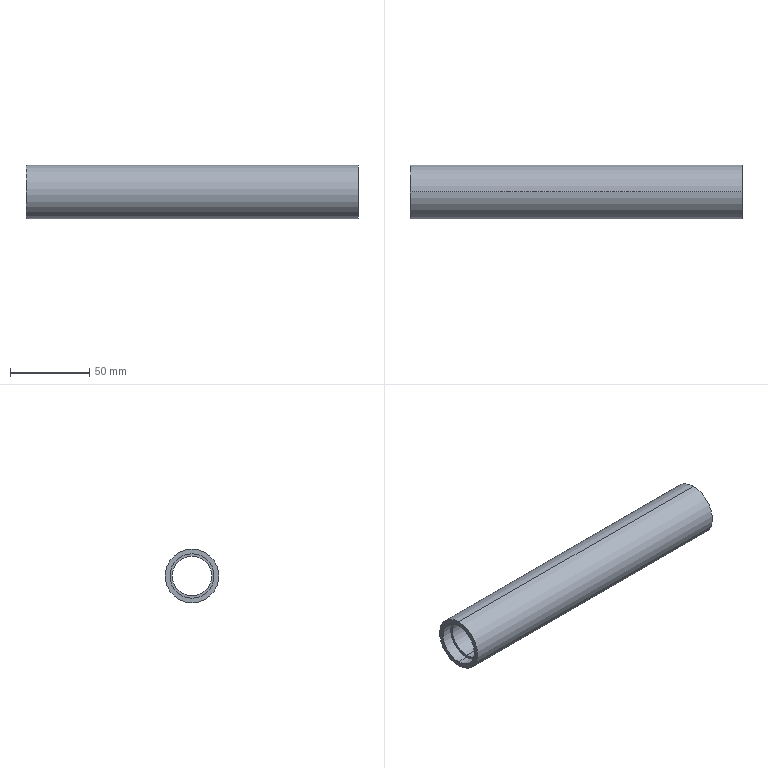Part | SolidWorks | features Revolution 1 | 1 solid | 12 faces | box 210 x 34 x 34 mm | volume 85831 mm3 | cylinder 8 | plane 4 | commonest cylinder face diameters 28 x4 25 x2 34 x2
STEP:
#1=CARTESIAN_POINT('',(98.,0.,-12.5));
#2=VERTEX_POINT('',#1);
#3=CARTESIAN_POINT('',(98.,0.,12.5));
#4=VERTEX_POINT('',#3);
#5=CARTESIAN_POINT('',(98.,0.,0.));
#6=DIRECTION('',(-1.,0.,0.));
#7=DIRECTION('',(0.,0.,1.));
#8=AXIS2_PLACEMENT_3D('',#5,#6,#7);
#9=CIRCLE('',#8,12.5);
#10=EDGE_CURVE('',#2,#4,#9,.T.);
#11=ORIENTED_EDGE('',*,*,#10,.F.);
#12=CARTESIAN_POINT('',(-98.,0.,-12.5));
#13=VERTEX_POINT('',#12);
#14=CARTESIAN_POINT('',(0.,0.,-12.5));
#15=DIRECTION('',(-1.,0.,0.));
#16=VECTOR('',#15,1000.);
#17=LINE('',#14,#16);
#18=EDGE_CURVE('',#2,#13,#17,.T.);
#19=ORIENTED_EDGE('',*,*,#18,.T.);
#20=CARTESIAN_POINT('',(-98.,0.,12.5));
#21=VERTEX_POINT('',#20);
#22=CARTESIAN_POINT('',(-98.,0.,0.));
#23=DIRECTION('',(-1.,0.,0.));
#24=DIRECTION('',(0.,0.,1.));
#25=AXIS2_PLACEMENT_3D('',#22,#23,#24);
#26=CIRCLE('',#25,12.5);
#27=EDGE_CURVE('',#13,#21,#26,.T.);
#28=ORIENTED_EDGE('',*,*,#27,.T.);
#29=CARTESIAN_POINT('',(0.,0.,12.5));
#30=DIRECTION('',(-1.,0.,0.));
#31=VECTOR('',#30,1000.);
#32=LINE('',#29,#31);
#33=EDGE_CURVE('',#4,#21,#32,.T.);
#34=ORIENTED_EDGE('',*,*,#33,.F.);
#35=EDGE_LOOP('',(#11,#19,#28,#34));
#36=FACE_OUTER_BOUND('',#35,.T.);
#37=CARTESIAN_POINT('',(0.,0.,0.));
#38=DIRECTION('',(-1.,0.,0.));
#39=DIRECTION('',(0.,0.,1.));
#40=AXIS2_PLACEMENT_3D('',#37,#38,#39);
#41=CYLINDRICAL_SURFACE('',#40,12.5);
#42=ADVANCED_FACE('',(#36),#41,.F.);
#43=CARTESIAN_POINT('',(105.,0.,-14.));
#44=VERTEX_POINT('',#43);
#45=CARTESIAN_POINT('',(105.,0.,14.));
#46=VERTEX_POINT('',#45);
#47=CARTESIAN_POINT('',(105.,0.,0.));
#48=DIRECTION('',(-1.,0.,0.));
#49=DIRECTION('',(0.,0.,1.));
#50=AXIS2_PLACEMENT_3D('',#47,#48,#49);
#51=CIRCLE('',#50,14.);
#52=EDGE_CURVE('',#44,#46,#51,.T.);
#53=ORIENTED_EDGE('',*,*,#52,.F.);
#54=CARTESIAN_POINT('',(98.,0.,-14.));
#55=VERTEX_POINT('',#54);
#56=CARTESIAN_POINT('',(0.,0.,-14.));
#57=DIRECTION('',(-1.,0.,0.));
#58=VECTOR('',#57,1000.);
#59=LINE('',#56,#58);
#60=EDGE_CURVE('',#44,#55,#59,.T.);
#61=ORIENTED_EDGE('',*,*,#60,.T.);
#62=CARTESIAN_POINT('',(98.,0.,14.));
#63=VERTEX_POINT('',#62);
#64=CARTESIAN_POINT('',(98.,0.,0.));
#65=DIRECTION('',(-1.,0.,0.));
#66=DIRECTION('',(0.,0.,1.));
#67=AXIS2_PLACEMENT_3D('',#64,#65,#66);
#68=CIRCLE('',#67,14.);
#69=EDGE_CURVE('',#55,#63,#68,.T.);
#70=ORIENTED_EDGE('',*,*,#69,.T.);
#71=CARTESIAN_POINT('',(0.,0.,14.));
#72=DIRECTION('',(-1.,0.,0.));
#73=VECTOR('',#72,1000.);
#74=LINE('',#71,#73);
#75=EDGE_CURVE('',#46,#63,#74,.T.);
#76=ORIENTED_EDGE('',*,*,#75,.F.);
#77=EDGE_LOOP('',(#53,#61,#70,#76));
#78=FACE_OUTER_BOUND('',#77,.T.);
#79=CARTESIAN_POINT('',(0.,0.,0.));
#80=DIRECTION('',(-1.,0.,0.));
#81=DIRECTION('',(0.,0.,1.));
#82=AXIS2_PLACEMENT_3D('',#79,#80,#81);
#83=CYLINDRICAL_SURFACE('',#82,14.);
#84=ADVANCED_FACE('',(#78),#83,.F.);
#85=CARTESIAN_POINT('',(105.,0.,17.));
#86=VERTEX_POINT('',#85);
#87=CARTESIAN_POINT('',(105.,0.,-17.));
#88=VERTEX_POINT('',#87);
#89=CARTESIAN_POINT('',(105.,0.,0.));
#90=DIRECTION('',(-1.,0.,0.));
#91=DIRECTION('',(0.,0.,1.));
#92=AXIS2_PLACEMENT_3D('',#89,#90,#91);
#93=CIRCLE('',#92,17.);
#94=EDGE_CURVE('',#86,#88,#93,.T.);
#95=ORIENTED_EDGE('',*,*,#94,.T.);
#96=CARTESIAN_POINT('',(-105.,0.,-17.));
#97=VERTEX_POINT('',#96);
#98=CARTESIAN_POINT('',(0.,0.,-17.));
#99=DIRECTION('',(-1.,0.,0.));
#100=VECTOR('',#99,1000.);
#101=LINE('',#98,#100);
#102=EDGE_CURVE('',#88,#97,#101,.T.);
#103=ORIENTED_EDGE('',*,*,#102,.T.);
#104=CARTESIAN_POINT('',(-105.,0.,17.));
#105=VERTEX_POINT('',#104);
#106=CARTESIAN_POINT('',(-105.,0.,0.));
#107=DIRECTION('',(-1.,0.,0.));
#108=DIRECTION('',(0.,0.,1.));
#109=AXIS2_PLACEMENT_3D('',#106,#107,#108);
#110=CIRCLE('',#109,17.);
#111=EDGE_CURVE('',#105,#97,#110,.T.);
#112=ORIENTED_EDGE('',*,*,#111,.F.);
#113=CARTESIAN_POINT('',(0.,0.,17.));
#114=DIRECTION('',(-1.,0.,0.));
#115=VECTOR('',#114,1000.);
#116=LINE('',#113,#115);
#117=EDGE_CURVE('',#86,#105,#116,.T.);
#118=ORIENTED_EDGE('',*,*,#117,.F.);
#119=EDGE_LOOP('',(#95,#103,#112,#118));
#120=FACE_OUTER_BOUND('',#119,.T.);
#121=CARTESIAN_POINT('',(0.,0.,0.));
#122=DIRECTION('',(-1.,0.,0.));
#123=DIRECTION('',(0.,0.,1.));
#124=AXIS2_PLACEMENT_3D('',#121,#122,#123);
#125=CYLINDRICAL_SURFACE('',#124,17.);
#126=ADVANCED_FACE('',(#120),#125,.T.);
#127=CARTESIAN_POINT('',(-98.,0.,-14.));
#128=VERTEX_POINT('',#127);
#129=CARTESIAN_POINT('',(-98.,0.,14.));
#130=VERTEX_POINT('',#129);
#131=CARTESIAN_POINT('',(-98.,0.,0.));
#132=DIRECTION('',(-1.,0.,0.));
#133=DIRECTION('',(0.,0.,1.));
#134=AXIS2_PLACEMENT_3D('',#131,#132,#133);
#135=CIRCLE('',#134,14.);
#136=EDGE_CURVE('',#128,#130,#135,.T.);
#137=ORIENTED_EDGE('',*,*,#136,.F.);
#138=CARTESIAN_POINT('',(-105.,0.,-14.));
#139=VERTEX_POINT('',#138);
#140=CARTESIAN_POINT('',(0.,0.,-14.));
#141=DIRECTION('',(-1.,0.,0.));
#142=VECTOR('',#141,1000.);
#143=LINE('',#140,#142);
#144=EDGE_CURVE('',#128,#139,#143,.T.);
#145=ORIENTED_EDGE('',*,*,#144,.T.);
#146=CARTESIAN_POINT('',(-105.,0.,14.));
#147=VERTEX_POINT('',#146);
#148=CARTESIAN_POINT('',(-105.,0.,0.));
#149=DIRECTION('',(-1.,0.,0.));
#150=DIRECTION('',(0.,0.,1.));
#151=AXIS2_PLACEMENT_3D('',#148,#149,#150);
#152=CIRCLE('',#151,14.);
#153=EDGE_CURVE('',#139,#147,#152,.T.);
#154=ORIENTED_EDGE('',*,*,#153,.T.);
#155=CARTESIAN_POINT('',(0.,0.,14.));
#156=DIRECTION('',(-1.,0.,0.));
#157=VECTOR('',#156,1000.);
#158=LINE('',#155,#157);
#159=EDGE_CURVE('',#130,#147,#158,.T.);
#160=ORIENTED_EDGE('',*,*,#159,.F.);
#161=EDGE_LOOP('',(#137,#145,#154,#160));
#162=FACE_OUTER_BOUND('',#161,.T.);
#163=CARTESIAN_POINT('',(0.,0.,0.));
#164=DIRECTION('',(-1.,0.,0.));
#165=DIRECTION('',(0.,0.,1.));
#166=AXIS2_PLACEMENT_3D('',#163,#164,#165);
#167=CYLINDRICAL_SURFACE('',#166,14.);
#168=ADVANCED_FACE('',(#162),#167,.F.);
#169=ORIENTED_EDGE('',*,*,#144,.F.);
#170=CARTESIAN_POINT('',(-98.,0.,0.));
#171=DIRECTION('',(-1.,0.,0.));
#172=DIRECTION('',(0.,0.,1.));
#173=AXIS2_PLACEMENT_3D('',#170,#171,#172);
#174=CIRCLE('',#173,14.);
#175=EDGE_CURVE('',#130,#128,#174,.T.);
#176=ORIENTED_EDGE('',*,*,#175,.F.);
#177=ORIENTED_EDGE('',*,*,#159,.T.);
#178=CARTESIAN_POINT('',(-105.,0.,0.));
#179=DIRECTION('',(-1.,0.,0.));
#180=DIRECTION('',(0.,0.,1.));
#181=AXIS2_PLACEMENT_3D('',#178,#179,#180);
#182=CIRCLE('',#181,14.);
#183=EDGE_CURVE('',#147,#139,#182,.T.);
#184=ORIENTED_EDGE('',*,*,#183,.T.);
#185=EDGE_LOOP('',(#169,#176,#177,#184));
#186=FACE_OUTER_BOUND('',#185,.T.);
#187=CARTESIAN_POINT('',(0.,0.,0.));
#188=DIRECTION('',(-1.,0.,0.));
#189=DIRECTION('',(0.,0.,1.));
#190=AXIS2_PLACEMENT_3D('',#187,#188,#189);
#191=CYLINDRICAL_SURFACE('',#190,14.);
#192=ADVANCED_FACE('',(#186),#191,.F.);
#193=ORIENTED_EDGE('',*,*,#183,.F.);
#194=ORIENTED_EDGE('',*,*,#153,.F.);
#195=EDGE_LOOP('',(#193,#194));
#196=FACE_BOUND('',#195,.T.);
#197=ORIENTED_EDGE('',*,*,#111,.T.);
#198=CARTESIAN_POINT('',(-105.,0.,0.));
#199=DIRECTION('',(-1.,0.,0.));
#200=DIRECTION('',(0.,0.,1.));
#201=AXIS2_PLACEMENT_3D('',#198,#199,#200);
#202=CIRCLE('',#201,17.);
#203=EDGE_CURVE('',#97,#105,#202,.T.);
#204=ORIENTED_EDGE('',*,*,#203,.T.);
#205=EDGE_LOOP('',(#197,#204));
#206=FACE_OUTER_BOUND('',#205,.T.);
#207=CARTESIAN_POINT('',(-105.,17.,0.));
#208=DIRECTION('',(1.,0.,0.));
#209=DIRECTION('',(0.,0.,-1.));
#210=AXIS2_PLACEMENT_3D('',#207,#208,#209);
#211=PLANE('',#210);
#212=ADVANCED_FACE('',(#196,#206),#211,.F.);
#213=ORIENTED_EDGE('',*,*,#102,.F.);
#214=CARTESIAN_POINT('',(105.,0.,0.));
#215=DIRECTION('',(-1.,0.,0.));
#216=DIRECTION('',(0.,0.,1.));
#217=AXIS2_PLACEMENT_3D('',#214,#215,#216);
#218=CIRCLE('',#217,17.);
#219=EDGE_CURVE('',#88,#86,#218,.T.);
#220=ORIENTED_EDGE('',*,*,#219,.T.);
#221=ORIENTED_EDGE('',*,*,#117,.T.);
#222=ORIENTED_EDGE('',*,*,#203,.F.);
#223=EDGE_LOOP('',(#213,#220,#221,#222));
#224=FACE_OUTER_BOUND('',#223,.T.);
#225=CARTESIAN_POINT('',(0.,0.,0.));
#226=DIRECTION('',(-1.,0.,0.));
#227=DIRECTION('',(0.,0.,1.));
#228=AXIS2_PLACEMENT_3D('',#225,#226,#227);
#229=CYLINDRICAL_SURFACE('',#228,17.);
#230=ADVANCED_FACE('',(#224),#229,.T.);
#231=ORIENTED_EDGE('',*,*,#94,.F.);
#232=ORIENTED_EDGE('',*,*,#219,.F.);
#233=EDGE_LOOP('',(#231,#232));
#234=FACE_OUTER_BOUND('',#233,.T.);
#235=CARTESIAN_POINT('',(105.,0.,0.));
#236=DIRECTION('',(-1.,0.,0.));
#237=DIRECTION('',(0.,0.,1.));
#238=AXIS2_PLACEMENT_3D('',#235,#236,#237);
#239=CIRCLE('',#238,14.);
#240=EDGE_CURVE('',#46,#44,#239,.T.);
#241=ORIENTED_EDGE('',*,*,#240,.T.);
#242=ORIENTED_EDGE('',*,*,#52,.T.);
#243=EDGE_LOOP('',(#241,#242));
#244=FACE_BOUND('',#243,.T.);
#245=CARTESIAN_POINT('',(105.,17.,0.));
#246=DIRECTION('',(-1.,0.,0.));
#247=DIRECTION('',(0.,0.,1.));
#248=AXIS2_PLACEMENT_3D('',#245,#246,#247);
#249=PLANE('',#248);
#250=ADVANCED_FACE('',(#234,#244),#249,.F.);
#251=ORIENTED_EDGE('',*,*,#60,.F.);
#252=ORIENTED_EDGE('',*,*,#240,.F.);
#253=ORIENTED_EDGE('',*,*,#75,.T.);
#254=CARTESIAN_POINT('',(98.,0.,0.));
#255=DIRECTION('',(-1.,0.,0.));
#256=DIRECTION('',(0.,0.,1.));
#257=AXIS2_PLACEMENT_3D('',#254,#255,#256);
#258=CIRCLE('',#257,14.);
#259=EDGE_CURVE('',#63,#55,#258,.T.);
#260=ORIENTED_EDGE('',*,*,#259,.T.);
#261=EDGE_LOOP('',(#251,#252,#253,#260));
#262=FACE_OUTER_BOUND('',#261,.T.);
#263=CARTESIAN_POINT('',(0.,0.,0.));
#264=DIRECTION('',(-1.,0.,0.));
#265=DIRECTION('',(0.,0.,1.));
#266=AXIS2_PLACEMENT_3D('',#263,#264,#265);
#267=CYLINDRICAL_SURFACE('',#266,14.);
#268=ADVANCED_FACE('',(#262),#267,.F.);
#269=ORIENTED_EDGE('',*,*,#259,.F.);
#270=ORIENTED_EDGE('',*,*,#69,.F.);
#271=EDGE_LOOP('',(#269,#270));
#272=FACE_OUTER_BOUND('',#271,.T.);
#273=CARTESIAN_POINT('',(98.,0.,0.));
#274=DIRECTION('',(-1.,0.,0.));
#275=DIRECTION('',(0.,0.,1.));
#276=AXIS2_PLACEMENT_3D('',#273,#274,#275);
#277=CIRCLE('',#276,12.5);
#278=EDGE_CURVE('',#4,#2,#277,.T.);
#279=ORIENTED_EDGE('',*,*,#278,.T.);
#280=ORIENTED_EDGE('',*,*,#10,.T.);
#281=EDGE_LOOP('',(#279,#280));
#282=FACE_BOUND('',#281,.T.);
#283=CARTESIAN_POINT('',(98.,14.,0.));
#284=DIRECTION('',(-1.,0.,0.));
#285=DIRECTION('',(0.,0.,1.));
#286=AXIS2_PLACEMENT_3D('',#283,#284,#285);
#287=PLANE('',#286);
#288=ADVANCED_FACE('',(#272,#282),#287,.F.);
#289=ORIENTED_EDGE('',*,*,#18,.F.);
#290=ORIENTED_EDGE('',*,*,#278,.F.);
#291=ORIENTED_EDGE('',*,*,#33,.T.);
#292=CARTESIAN_POINT('',(-98.,0.,0.));
#293=DIRECTION('',(-1.,0.,0.));
#294=DIRECTION('',(0.,0.,1.));
#295=AXIS2_PLACEMENT_3D('',#292,#293,#294);
#296=CIRCLE('',#295,12.5);
#297=EDGE_CURVE('',#21,#13,#296,.T.);
#298=ORIENTED_EDGE('',*,*,#297,.T.);
#299=EDGE_LOOP('',(#289,#290,#291,#298));
#300=FACE_OUTER_BOUND('',#299,.T.);
#301=CARTESIAN_POINT('',(0.,0.,0.));
#302=DIRECTION('',(-1.,0.,0.));
#303=DIRECTION('',(0.,0.,1.));
#304=AXIS2_PLACEMENT_3D('',#301,#302,#303);
#305=CYLINDRICAL_SURFACE('',#304,12.5);
#306=ADVANCED_FACE('',(#300),#305,.F.);
#307=ORIENTED_EDGE('',*,*,#297,.F.);
#308=ORIENTED_EDGE('',*,*,#27,.F.);
#309=EDGE_LOOP('',(#307,#308));
#310=FACE_BOUND('',#309,.T.);
#311=ORIENTED_EDGE('',*,*,#175,.T.);
#312=ORIENTED_EDGE('',*,*,#136,.T.);
#313=EDGE_LOOP('',(#311,#312));
#314=FACE_OUTER_BOUND('',#313,.T.);
#315=CARTESIAN_POINT('',(-98.,14.,0.));
#316=DIRECTION('',(1.,0.,0.));
#317=DIRECTION('',(0.,0.,-1.));
#318=AXIS2_PLACEMENT_3D('',#315,#316,#317);
#319=PLANE('',#318);
#320=ADVANCED_FACE('',(#310,#314),#319,.F.);
#321=CLOSED_SHELL('',(#42,#84,#126,#168,#192,#212,#230,#250,#268,#288,#306,#320));
#322=MANIFOLD_SOLID_BREP('',#321);
#323=CARTESIAN_POINT('',(0.,0.,0.));
#324=DIRECTION('',(0.,0.,1.));
#325=DIRECTION('',(1.,0.,0.));
#326=AXIS2_PLACEMENT_3D('',#323,#324,#325);
#327=(LENGTH_UNIT()NAMED_UNIT(*)SI_UNIT(.MILLI.,.METRE.));
#328=UNCERTAINTY_MEASURE_WITH_UNIT(LENGTH_MEASURE(0.00001),#327,'','');
#329=(NAMED_UNIT(*)PLANE_ANGLE_UNIT()SI_UNIT($,.RADIAN.));
#330=(NAMED_UNIT(*)SI_UNIT($,.STERADIAN.)SOLID_ANGLE_UNIT());
#331=(GEOMETRIC_REPRESENTATION_CONTEXT(3)GLOBAL_UNCERTAINTY_ASSIGNED_CONTEXT((#328))GLOBAL_UNIT_ASSIGNED_CONTEXT((#327,#329,#330))REPRESENTATION_CONTEXT('',''));
#332=ADVANCED_BREP_SHAPE_REPRESENTATION('',(#322,#326),#331);